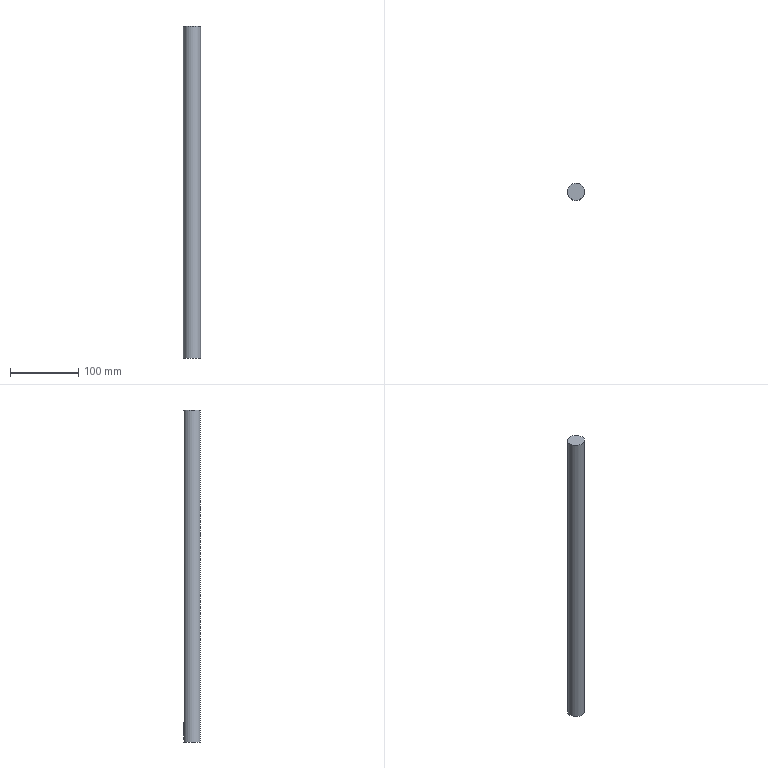NC program | NX | posted with a generic post | part box 25 x 25 x 487 mm
Whole program:
N10 G17 G21 G94 G90
(ZLEVEL_PROFILE , TOOL : D6)
N12 T06 M6
N14 G54
N16 G17 G0 G90 X-15.354 Y0.9 B0. C0. S3800 M3
N18 G43 Z70. H6
N20 Z1.
N22 G94 G1 X-24.885 Z0.501 F1000.
N24 X-25.139 Y0.823 Z0.487
N26 X-25.359 Y0.676 Z0.473
N28 X-25.529 Y0.471 Z0.459
N30 X-25.632 Y0.223 Z0.445
N32 X-25.647 Y-0.154 Z0.425
N34 X-25.507 Y-0.504 Z0.405
N36 X-25.238 Y-0.768 Z0.385
N38 X-24.885 Y-0.9 Z0.366
N40 X-16. Z-0.1
N42 X-7.25 F1650.
N44 G3 X-6.35 Y0. R0.9
N46 X-7.25 Y0.9 R0.9
N48 G1 X-24.75
N50 G3 X-25.65 Y0. R0.9
N52 X-24.75 Y-0.9 R0.9
N54 G1 X-16.
N56 X-10.271 Z-0.2
N58 X-7.25
N60 G3 X-6.35 Y0. R0.9
N62 X-7.25 Y0.9 R0.9
N64 G1 X-24.75
N66 G3 X-25.65 Y0. R0.9
N68 X-24.75 Y-0.9 R0.9
N70 G1 X-16.
N72 X-10.271 Z-0.3
N74 X-7.25
N76 G3 X-6.35 Y0. R0.9
N78 X-7.25 Y0.9 R0.9
N80 G1 X-24.75
N82 G3 X-25.65 Y0. R0.9
N84 X-24.75 Y-0.9 R0.9
N86 G1 X-16.
N88 X-10.271 Z-0.4
N90 X-7.25
N92 G3 X-6.35 Y0. R0.9
N94 X-7.25 Y0.9 R0.9
N96 G1 X-24.75
N98 G3 X-25.65 Y0. R0.9
N100 X-24.75 Y-0.9 R0.9
N102 G1 X-16.
N104 X-10.271 Z-0.5
N106 X-7.25
N108 G3 X-6.35 Y0. R0.9
N110 X-7.25 Y0.9 R0.9
N112 G1 X-24.75
N114 G3 X-25.65 Y0. R0.9
N116 X-24.75 Y-0.9 R0.9
N118 G1 X-16.
N120 X-10.271 Z-0.6
N122 X-7.25
N124 G3 X-6.35 Y0. R0.9
N126 X-7.25 Y0.9 R0.9
N128 G1 X-24.75
N130 G3 X-25.65 Y0. R0.9
N132 X-24.75 Y-0.9 R0.9
N134 G1 X-16.
N136 X-10.271 Z-0.7
N138 X-7.25
N140 G3 X-6.35 Y0. R0.9
N142 X-7.25 Y0.9 R0.9
N144 G1 X-24.75
N146 G3 X-25.65 Y0. R0.9
N148 X-24.75 Y-0.9 R0.9
N150 G1 X-16.
N152 X-10.271 Z-0.8
N154 X-7.25
N156 G3 X-6.35 Y0. R0.9
N158 X-7.25 Y0.9 R0.9
N160 G1 X-24.75
N162 G3 X-25.65 Y0. R0.9
N164 X-24.75 Y-0.9 R0.9
N166 G1 X-16.
N168 X-10.271 Z-0.9
N170 X-7.25
N172 G3 X-6.35 Y0. R0.9
N174 X-7.25 Y0.9 R0.9
N176 G1 X-24.75
N178 G3 X-25.65 Y0. R0.9
N180 X-24.75 Y-0.9 R0.9
N182 G1 X-16.
N184 X-10.271 Z-1.
N186 X-7.25
N188 G3 X-6.35 Y0. R0.9
N190 X-7.25 Y0.9 R0.9
N192 G1 X-24.75
N194 G3 X-25.65 Y0. R0.9
N196 X-24.75 Y-0.9 R0.9
N198 G1 X-16.
N200 X-10.271 Z-1.1
N202 X-7.25
N204 G3 X-6.35 Y0. R0.9
N206 X-7.25 Y0.9 R0.9
N208 G1 X-24.75
N210 G3 X-25.65 Y0. R0.9
N212 X-24.75 Y-0.9 R0.9
N214 G1 X-16.
N216 X-10.271 Z-1.2
N218 X-7.25
N220 G3 X-6.35 Y0. R0.9
N222 X-7.25 Y0.9 R0.9
N224 G1 X-24.75
N226 G3 X-25.65 Y0. R0.9
N228 X-24.75 Y-0.9 R0.9
N230 G1 X-16.
N232 X-10.271 Z-1.3
N234 X-7.25
N236 G3 X-6.35 Y0. R0.9
N238 X-7.25 Y0.9 R0.9
N240 G1 X-24.75
N242 G3 X-25.65 Y0. R0.9
N244 X-24.75 Y-0.9 R0.9
N246 G1 X-16.
N248 X-10.271 Z-1.4
N250 X-7.25
N252 G3 X-6.35 Y0. R0.9
N254 X-7.25 Y0.9 R0.9
N256 G1 X-24.75
N258 G3 X-25.65 Y0. R0.9
N260 X-24.75 Y-0.9 R0.9
N262 G1 X-16.
N264 X-10.271 Z-1.5
N266 X-7.25
N268 G3 X-6.35 Y0. R0.9
N270 X-7.25 Y0.9 R0.9
N272 G1 X-24.75
N274 G3 X-25.65 Y0. R0.9
N276 X-24.75 Y-0.9 R0.9
N278 G1 X-16.
N280 X-10.271 Z-1.6
N282 X-7.25
N284 G3 X-6.35 Y0. R0.9
N286 X-7.25 Y0.9 R0.9
N288 G1 X-24.75
N290 G3 X-25.65 Y0. R0.9
N292 X-24.75 Y-0.9 R0.9
N294 G1 X-16.
N296 X-10.271 Z-1.7
N298 X-7.25
N300 G3 X-6.35 Y0. R0.9
N302 X-7.25 Y0.9 R0.9
N304 G1 X-24.75
N306 G3 X-25.65 Y0. R0.9
N308 X-24.75 Y-0.9 R0.9
N310 G1 X-16.
N312 X-10.271 Z-1.8
N314 X-7.25
N316 G3 X-6.35 Y0. R0.9
N318 X-7.25 Y0.9 R0.9
N320 G1 X-24.75
N322 G3 X-25.65 Y0. R0.9
N324 X-24.75 Y-0.9 R0.9
N326 G1 X-16.
N328 X-10.271 Z-1.9
N330 X-7.25
N332 G3 X-6.35 Y0. R0.9
N334 X-7.25 Y0.9 R0.9
N336 G1 X-24.75
N338 G3 X-25.65 Y0. R0.9
N340 X-24.75 Y-0.9 R0.9
N342 G1 X-16.
N344 X-10.271 Z-2.
N346 X-7.25
N348 G3 X-6.35 Y0. R0.9
N350 X-7.25 Y0.9 R0.9
N352 G1 X-24.75
N354 G3 X-25.65 Y0. R0.9
N356 X-24.75 Y-0.9 R0.9
N358 G1 X-16.
N360 X-10.271 Z-2.1
N362 X-7.25
N364 G3 X-6.35 Y0. R0.9
N366 X-7.25 Y0.9 R0.9
N368 G1 X-24.75
N370 G3 X-25.65 Y0. R0.9
N372 X-24.75 Y-0.9 R0.9
N374 G1 X-16.
N376 X-10.271 Z-2.2
N378 X-7.25
N380 G3 X-6.35 Y0. R0.9
N382 X-7.25 Y0.9 R0.9
N384 G1 X-24.75
N386 G3 X-25.65 Y0. R0.9
N388 X-24.75 Y-0.9 R0.9
N390 G1 X-16.
N392 X-10.271 Z-2.3
N394 X-7.25
N396 G3 X-6.35 Y0. R0.9
N398 X-7.25 Y0.9 R0.9
N400 G1 X-24.75
N402 G3 X-25.65 Y0. R0.9
N404 X-24.75 Y-0.9 R0.9
N406 G1 X-16.
N408 X-10.271 Z-2.4
N410 X-7.25
N412 G3 X-6.35 Y0. R0.9
N414 X-7.25 Y0.9 R0.9
N416 G1 X-24.75
N418 G3 X-25.65 Y0. R0.9
N420 X-24.75 Y-0.9 R0.9
N422 G1 X-16.
N424 X-10.271 Z-2.5
N426 X-7.25
N428 G3 X-6.35 Y0. R0.9
N430 X-7.25 Y0.9 R0.9
N432 G1 X-24.75
N434 G3 X-25.65 Y0. R0.9
N436 X-24.75 Y-0.9 R0.9
N438 G1 X-16.
N440 X-10.271 Z-2.6
N442 X-7.25
N444 G3 X-6.35 Y0. R0.9
N446 X-7.25 Y0.9 R0.9
N448 G1 X-24.75
N450 G3 X-25.65 Y0. R0.9
N452 X-24.75 Y-0.9 R0.9
N454 G1 X-16.
N456 X-10.271 Z-2.7
N458 X-7.25
N460 G3 X-6.35 Y0. R0.9
N462 X-7.25 Y0.9 R0.9
N464 G1 X-24.75
N466 G3 X-25.65 Y0. R0.9
N468 X-24.75 Y-0.9 R0.9
N470 G1 X-16.
N472 X-10.271 Z-2.8
N474 X-7.25
N476 G3 X-6.35 Y0. R0.9
N478 X-7.25 Y0.9 R0.9
N480 G1 X-24.75
N482 G3 X-25.65 Y0. R0.9
N484 X-24.75 Y-0.9 R0.9
N486 G1 X-16.
N488 X-10.271 Z-2.9
N490 X-7.25
N492 G3 X-6.35 Y0. R0.9
N494 X-7.25 Y0.9 R0.9
N496 G1 X-24.75
N498 G3 X-25.65 Y0. R0.9
N500 X-24.75 Y-0.9 R0.9
N502 G1 X-16.
N504 X-10.271 Z-3.
N506 X-7.25
N508 G3 X-6.35 Y0. R0.9
N510 X-7.25 Y0.9 R0.9
N512 G1 X-24.75
N514 G3 X-25.65 Y0. R0.9
N516 X-24.75 Y-0.9 R0.9
N518 G1 X-16.
N520 X-10.271 Z-3.1
N522 X-7.25
N524 G3 X-6.35 Y0. R0.9
N526 X-7.25 Y0.9 R0.9
N528 G1 X-24.75
N530 G3 X-25.65 Y0. R0.9
N532 X-24.75 Y-0.9 R0.9
N534 G1 X-16.
N536 X-10.271 Z-3.2
N538 X-7.25
N540 G3 X-6.35 Y0. R0.9
N542 X-7.25 Y0.9 R0.9
N544 G1 X-24.75
N546 G3 X-25.65 Y0. R0.9
N548 X-24.75 Y-0.9 R0.9
N550 G1 X-16.
N552 X-10.271 Z-3.3
N554 X-7.25
N556 G3 X-6.35 Y0. R0.9
N558 X-7.25 Y0.9 R0.9
N560 G1 X-24.75
N562 G3 X-25.65 Y0. R0.9
N564 X-24.75 Y-0.9 R0.9
N566 G1 X-16.
N568 X-10.271 Z-3.4
N570 X-7.25
N572 G3 X-6.35 Y0. R0.9
N574 X-7.25 Y0.9 R0.9
N576 G1 X-24.75
N578 G3 X-25.65 Y0. R0.9
N580 X-24.75 Y-0.9 R0.9
N582 G1 X-16.
N584 X-10.271 Z-3.5
N586 X-7.25
N588 G3 X-6.35 Y0. R0.9
N590 X-7.25 Y0.9 R0.9
N592 G1 X-24.75
N594 G3 X-25.65 Y0. R0.9
N596 X-24.75 Y-0.9 R0.9
N598 G1 X-16.
N600 X-10.271 Z-3.6
N602 X-7.25
N604 G3 X-6.35 Y0. R0.9
N606 X-7.25 Y0.9 R0.9
N608 G1 X-24.75
N610 G3 X-25.65 Y0. R0.9
N612 X-24.75 Y-0.9 R0.9
N614 G1 X-16.
N616 X-10.271 Z-3.7
N618 X-7.25
N620 G3 X-6.35 Y0. R0.9
N622 X-7.25 Y0.9 R0.9
N624 G1 X-24.75
N626 G3 X-25.65 Y0. R0.9
N628 X-24.75 Y-0.9 R0.9
N630 G1 X-16.
N632 X-10.271 Z-3.8
N634 X-7.25
N636 G3 X-6.35 Y0. R0.9
N638 X-7.25 Y0.9 R0.9
N640 G1 X-24.75
N642 G3 X-25.65 Y0. R0.9
N644 X-24.75 Y-0.9 R0.9
N646 G1 X-16.
N648 X-10.271 Z-3.9
N650 X-7.25
N652 G3 X-6.35 Y0. R0.9
N654 X-7.25 Y0.9 R0.9
N656 G1 X-24.75
N658 G3 X-25.65 Y0. R0.9
N660 X-24.75 Y-0.9 R0.9
N662 G1 X-16.
N664 X-10.271 Z-4.
N666 X-7.25
N668 G3 X-6.35 Y0. R0.9
N670 X-7.25 Y0.9 R0.9
N672 G1 X-24.75
N674 G3 X-25.65 Y0. R0.9
N676 X-24.75 Y-0.9 R0.9
N678 G1 X-16.
N680 X-10.271 Z-4.1
N682 X-7.25
N684 G3 X-6.35 Y0. R0.9
N686 X-7.25 Y0.9 R0.9
N688 G1 X-24.75
N690 G3 X-25.65 Y0. R0.9
N692 X-24.75 Y-0.9 R0.9
N694 G1 X-16.
N696 X-10.271 Z-4.2
N698 X-7.25
N700 G3 X-6.35 Y0. R0.9
N702 X-7.25 Y0.9 R0.9
N704 G1 X-24.75
N706 G3 X-25.65 Y0. R0.9
N708 X-24.75 Y-0.9 R0.9
N710 G1 X-16.
N712 X-10.271 Z-4.3
N714 X-7.25
N716 G3 X-6.35 Y0. R0.9
N718 X-7.25 Y0.9 R0.9
N720 G1 X-24.75
N722 G3 X-25.65 Y0. R0.9
N724 X-24.75 Y-0.9 R0.9
N726 G1 X-16.
N728 X-10.271 Z-4.4
N730 X-7.25
N732 G3 X-6.35 Y0. R0.9
N734 X-7.25 Y0.9 R0.9
N736 G1 X-24.75
N738 G3 X-25.65 Y0. R0.9
N740 X-24.75 Y-0.9 R0.9
N742 G1 X-10.271
N744 Z-3.4
N746 G0 Z70.
N748 M5
(PROFILE_3D , TOOL : D6A45)
N750 T07 M6
N752 G54
N754 G17 G0 G90 X-23.863 Y2. B0. C0. S7000 M3
N756 G43 Z70. H7
N758 Z-1.156
N760 G94 G1 Z-2.156 F1250.
N762 X-24.125 Y2.358
N764 G3 X-24.674 Y2.6 R0.6
N766 G1 X-25.322 Y2.529 Z-2.117
N768 X-25.861 Y2.347 Z-1.999
N770 X-26.339 Y2.056 Z-1.883
N772 X-26.741 Y1.667 Z-1.751
N774 X-27.053 Y1.193 Z-1.617
N776 X-27.263 Y0.642 Z-1.553
N778 X-27.335 Y0.219 Z-1.507
N780 X-27.334 Y-0.226 Z-1.534
N782 X-27.257 Y-0.665 Z-1.561
N784 X-27.106 Y-1.084 Z-1.656
N786 X-26.888 Y-1.47 Z-1.75
N788 X-26.615 Y-1.803 Z-1.842
N790 X-26.214 Y-2.14 Z-1.953
N792 X-25.761 Y-2.388 Z-2.063
N794 X-25.268 Y-2.541 Z-2.107
N796 X-24.68 Y-2.6 Z-2.156
N798 X-7.33 Z-2.155
N800 X-6.659 Y-2.523 Z-2.11
N802 X-6.105 Y-2.325 Z-1.983
N804 X-5.61 Y-2.006 Z-1.857
N806 X-5.2 Y-1.585 Z-1.731
N808 X-4.896 Y-1.081 Z-1.605
N810 X-4.712 Y-0.518 Z-1.556
N812 X-4.661 Y0.073 Z-1.508
N814 X-4.745 Y0.664 Z-1.579
N816 X-4.948 Y1.195 Z-1.646
N818 X-5.261 Y1.669 Z-1.783
N820 X-5.663 Y2.057 Z-1.919
N822 X-6.14 Y2.348 Z-2.054
N824 X-6.679 Y2.53 Z-2.133
N826 X-7.326 Y2.6 Z-2.156
N828 X-24.674
N830 G3 X-25.194 Y2.3 R0.6
N832 G1 X-25.452 Y1.852
N834 Z-1.156
N836 G0 Z70.
N838 M5
(CUTTERCOMP6 , TOOL : D6)
N840 T06 M6
N842 G54
N844 G17 G0 G90 X-16.609 Y-0.25 B0. C0. S4800 M3
N846 G43 Z70. H6
N848 Z-3.4
N850 G94 G1 Z-4.4 F1000.
N852 G41 Y-0.35 D6
N854 X-16.591 Y-0.454
N856 G3 X-16. Y-0.95 R0.6
N858 G1 X-7.25
N860 G3 X-6.3 Y0. R0.95
N862 X-7.25 Y0.95 R0.95
N864 G1 X-24.75
N866 G3 X-25.7 Y0. R0.95
N868 X-24.75 Y-0.95 R0.95
N870 G1 X-16.
N872 G3 X-15.409 Y-0.454 R0.6
N874 G1 X-15.391 Y-0.35
N876 G40
N878 Y-0.25
N880 Z-3.4
N882 G0 Z70.
N884 M5
N886 M2